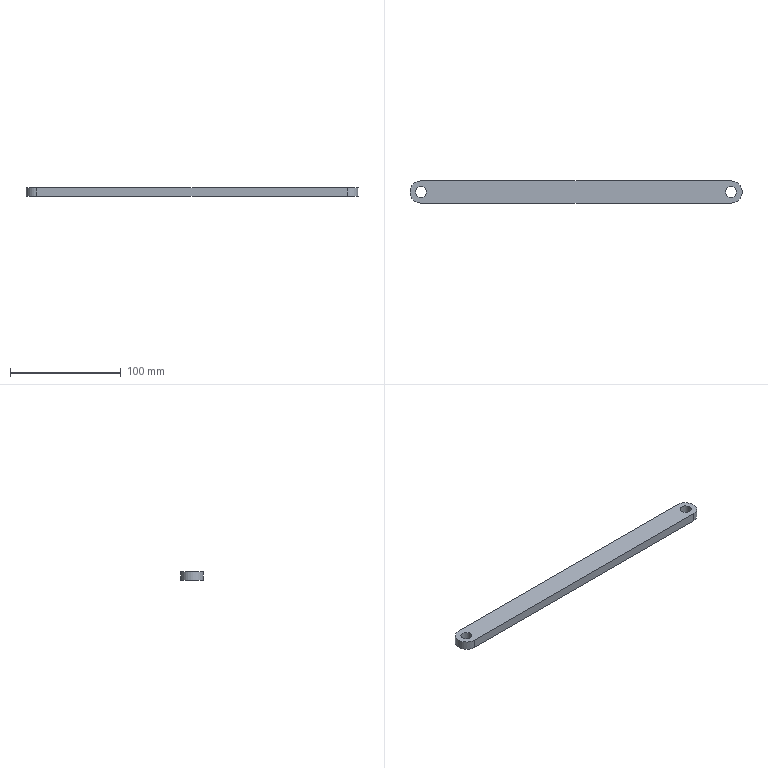Part | STEP file | tieqiangan | 1 solid | 8 faces | box 300 x 20 x 8 mm | volume 46057 mm3 | cylinder 4 | plane 4 | commonest cylinder face diameters 10 x2 20 x2
STEP:
#1=CARTESIAN_POINT('',(0.,0.,0.));
#2=DIRECTION('',(0.,0.,1.));
#3=DIRECTION('',(1.,0.,0.));
#4=AXIS2_PLACEMENT_3D('',#1,#2,#3);
#5=CARTESIAN_POINT('',(280.,10.,0.));
#6=VERTEX_POINT('',#5);
#7=CARTESIAN_POINT('',(280.,-10.,0.));
#8=VERTEX_POINT('',#7);
#9=CARTESIAN_POINT('',(280.,0.,0.));
#10=DIRECTION('',(0.,0.,-1.));
#11=DIRECTION('',(1.,0.,0.));
#12=AXIS2_PLACEMENT_3D('',#9,#10,#11);
#13=CIRCLE('',#12,10.);
#14=CARTESIAN_POINT('',(280.,0.,8.));
#15=DIRECTION('',(0.,0.,-1.));
#16=DIRECTION('',(-1.,0.,0.));
#17=AXIS2_PLACEMENT_3D('',#14,#15,#16);
#18=CYLINDRICAL_SURFACE('',#17,10.);
#19=CARTESIAN_POINT('',(-3.142,8.));
#20=DIRECTION('',(1.,0.));
#21=VECTOR('',#20,1.);
#22=LINE('',#19,#21);
#23=(GEOMETRIC_REPRESENTATION_CONTEXT(2)PARAMETRIC_REPRESENTATION_CONTEXT()REPRESENTATION_CONTEXT('',''));
#24=DEFINITIONAL_REPRESENTATION('',(#22),#23);
#25=PCURVE('',#18,#24);
#26=CARTESIAN_POINT('',(0.,0.,0.));
#27=DIRECTION('',(0.,0.,1.));
#28=DIRECTION('',(1.,0.,0.));
#29=AXIS2_PLACEMENT_3D('',#26,#27,#28);
#30=PLANE('',#29);
#31=CARTESIAN_POINT('',(290.,0.));
#32=CARTESIAN_POINT('',(290.,-17.321));
#33=CARTESIAN_POINT('',(275.,-8.66));
#34=CARTESIAN_POINT('',(260.,0.));
#35=CARTESIAN_POINT('',(275.,8.66));
#36=CARTESIAN_POINT('',(290.,17.321));
#37=CARTESIAN_POINT('',(290.,0.));
#38=(BOUNDED_CURVE()B_SPLINE_CURVE(2,(#31,#32,#33,#34,#35,#36,#37),.UNSPECIFIED.,.T.,.F.)B_SPLINE_CURVE_WITH_KNOTS((1,2,2,2,2,1),(-2.094,0.,2.094,4.189,6.283,8.378),.UNSPECIFIED.)CURVE()GEOMETRIC_REPRESENTATION_ITEM()RATIONAL_B_SPLINE_CURVE((1.,0.5,1.,0.5,1.,0.5,1.))REPRESENTATION_ITEM(''));
#39=(GEOMETRIC_REPRESENTATION_CONTEXT(2)PARAMETRIC_REPRESENTATION_CONTEXT()REPRESENTATION_CONTEXT('',''));
#40=DEFINITIONAL_REPRESENTATION('',(#38),#39);
#41=PCURVE('',#30,#40);
#42=SURFACE_CURVE('',#13,(#25,#41),.PCURVE_S1.);
#43=EDGE_CURVE('',#6,#8,#42,.T.);
#44=ORIENTED_EDGE('',*,*,#43,.F.);
#45=CARTESIAN_POINT('',(280.,10.,8.));
#46=VERTEX_POINT('',#45);
#47=CARTESIAN_POINT('',(280.,10.,8.));
#48=DIRECTION('',(0.,0.,-1.));
#49=VECTOR('',#48,1.);
#50=LINE('',#47,#49);
#51=CARTESIAN_POINT('',(1.571,0.));
#52=DIRECTION('',(0.,1.));
#53=VECTOR('',#52,1.);
#54=LINE('',#51,#53);
#55=(GEOMETRIC_REPRESENTATION_CONTEXT(2)PARAMETRIC_REPRESENTATION_CONTEXT()REPRESENTATION_CONTEXT('',''));
#56=DEFINITIONAL_REPRESENTATION('',(#54),#55);
#57=PCURVE('',#18,#56);
#58=CARTESIAN_POINT('',(0.,10.,8.));
#59=DIRECTION('',(0.,1.,0.));
#60=DIRECTION('',(-1.,0.,0.));
#61=AXIS2_PLACEMENT_3D('',#58,#59,#60);
#62=PLANE('',#61);
#63=CARTESIAN_POINT('',(-280.,0.));
#64=DIRECTION('',(0.,-1.));
#65=VECTOR('',#64,1.);
#66=LINE('',#63,#65);
#67=(GEOMETRIC_REPRESENTATION_CONTEXT(2)PARAMETRIC_REPRESENTATION_CONTEXT()REPRESENTATION_CONTEXT('',''));
#68=DEFINITIONAL_REPRESENTATION('',(#66),#67);
#69=PCURVE('',#62,#68);
#70=SURFACE_CURVE('',#50,(#57,#69),.PCURVE_S1.);
#71=EDGE_CURVE('',#46,#6,#70,.T.);
#72=ORIENTED_EDGE('',*,*,#71,.F.);
#73=CARTESIAN_POINT('',(280.,-10.,8.));
#74=VERTEX_POINT('',#73);
#75=CARTESIAN_POINT('',(280.,0.,8.));
#76=DIRECTION('',(0.,0.,-1.));
#77=DIRECTION('',(1.,0.,0.));
#78=AXIS2_PLACEMENT_3D('',#75,#76,#77);
#79=CIRCLE('',#78,10.);
#80=CARTESIAN_POINT('',(-3.142,0.));
#81=DIRECTION('',(1.,0.));
#82=VECTOR('',#81,1.);
#83=LINE('',#80,#82);
#84=(GEOMETRIC_REPRESENTATION_CONTEXT(2)PARAMETRIC_REPRESENTATION_CONTEXT()REPRESENTATION_CONTEXT('',''));
#85=DEFINITIONAL_REPRESENTATION('',(#83),#84);
#86=PCURVE('',#18,#85);
#87=CARTESIAN_POINT('',(0.,0.,8.));
#88=DIRECTION('',(0.,0.,1.));
#89=DIRECTION('',(1.,0.,0.));
#90=AXIS2_PLACEMENT_3D('',#87,#88,#89);
#91=PLANE('',#90);
#92=CARTESIAN_POINT('',(290.,0.));
#93=CARTESIAN_POINT('',(290.,-17.321));
#94=CARTESIAN_POINT('',(275.,-8.66));
#95=CARTESIAN_POINT('',(260.,0.));
#96=CARTESIAN_POINT('',(275.,8.66));
#97=CARTESIAN_POINT('',(290.,17.321));
#98=CARTESIAN_POINT('',(290.,0.));
#99=(BOUNDED_CURVE()B_SPLINE_CURVE(2,(#92,#93,#94,#95,#96,#97,#98),.UNSPECIFIED.,.T.,.F.)B_SPLINE_CURVE_WITH_KNOTS((1,2,2,2,2,1),(-2.094,0.,2.094,4.189,6.283,8.378),.UNSPECIFIED.)CURVE()GEOMETRIC_REPRESENTATION_ITEM()RATIONAL_B_SPLINE_CURVE((1.,0.5,1.,0.5,1.,0.5,1.))REPRESENTATION_ITEM(''));
#100=(GEOMETRIC_REPRESENTATION_CONTEXT(2)PARAMETRIC_REPRESENTATION_CONTEXT()REPRESENTATION_CONTEXT('',''));
#101=DEFINITIONAL_REPRESENTATION('',(#99),#100);
#102=PCURVE('',#91,#101);
#103=SURFACE_CURVE('',#79,(#86,#102),.PCURVE_S1.);
#104=EDGE_CURVE('',#46,#74,#103,.T.);
#105=ORIENTED_EDGE('',*,*,#104,.T.);
#106=CARTESIAN_POINT('',(280.,-10.,8.));
#107=DIRECTION('',(0.,0.,-1.));
#108=VECTOR('',#107,1.);
#109=LINE('',#106,#108);
#110=CARTESIAN_POINT('',(4.712,0.));
#111=DIRECTION('',(0.,1.));
#112=VECTOR('',#111,1.);
#113=LINE('',#110,#112);
#114=(GEOMETRIC_REPRESENTATION_CONTEXT(2)PARAMETRIC_REPRESENTATION_CONTEXT()REPRESENTATION_CONTEXT('',''));
#115=DEFINITIONAL_REPRESENTATION('',(#113),#114);
#116=PCURVE('',#18,#115);
#117=CARTESIAN_POINT('',(0.,-10.,8.));
#118=DIRECTION('',(0.,1.,0.));
#119=DIRECTION('',(-1.,0.,0.));
#120=AXIS2_PLACEMENT_3D('',#117,#118,#119);
#121=PLANE('',#120);
#122=CARTESIAN_POINT('',(-280.,0.));
#123=DIRECTION('',(0.,-1.));
#124=VECTOR('',#123,1.);
#125=LINE('',#122,#124);
#126=(GEOMETRIC_REPRESENTATION_CONTEXT(2)PARAMETRIC_REPRESENTATION_CONTEXT()REPRESENTATION_CONTEXT('',''));
#127=DEFINITIONAL_REPRESENTATION('',(#125),#126);
#128=PCURVE('',#121,#127);
#129=SURFACE_CURVE('',#109,(#116,#128),.PCURVE_S1.);
#130=EDGE_CURVE('',#74,#8,#129,.T.);
#131=ORIENTED_EDGE('',*,*,#130,.T.);
#132=EDGE_LOOP('',(#44,#72,#105,#131));
#133=FACE_BOUND('',#132,.T.);
#134=ADVANCED_FACE('',(#133),#18,.T.);
#135=CARTESIAN_POINT('',(0.,10.,0.));
#136=VERTEX_POINT('',#135);
#137=CARTESIAN_POINT('',(0.,10.,0.));
#138=DIRECTION('',(1.,0.,0.));
#139=VECTOR('',#138,1.);
#140=LINE('',#137,#139);
#141=CARTESIAN_POINT('',(0.,-8.));
#142=DIRECTION('',(-1.,0.));
#143=VECTOR('',#142,1.);
#144=LINE('',#141,#143);
#145=(GEOMETRIC_REPRESENTATION_CONTEXT(2)PARAMETRIC_REPRESENTATION_CONTEXT()REPRESENTATION_CONTEXT('',''));
#146=DEFINITIONAL_REPRESENTATION('',(#144),#145);
#147=PCURVE('',#62,#146);
#148=CARTESIAN_POINT('',(0.,10.));
#149=DIRECTION('',(1.,0.));
#150=VECTOR('',#149,1.);
#151=LINE('',#148,#150);
#152=(GEOMETRIC_REPRESENTATION_CONTEXT(2)PARAMETRIC_REPRESENTATION_CONTEXT()REPRESENTATION_CONTEXT('',''));
#153=DEFINITIONAL_REPRESENTATION('',(#151),#152);
#154=PCURVE('',#30,#153);
#155=SURFACE_CURVE('',#140,(#147,#154),.PCURVE_S1.);
#156=EDGE_CURVE('',#136,#6,#155,.T.);
#157=ORIENTED_EDGE('',*,*,#156,.F.);
#158=CARTESIAN_POINT('',(0.,10.,8.));
#159=VERTEX_POINT('',#158);
#160=CARTESIAN_POINT('',(0.,10.,8.));
#161=DIRECTION('',(0.,0.,-1.));
#162=VECTOR('',#161,1.);
#163=LINE('',#160,#162);
#164=CARTESIAN_POINT('',(0.,0.));
#165=DIRECTION('',(0.,-1.));
#166=VECTOR('',#165,1.);
#167=LINE('',#164,#166);
#168=(GEOMETRIC_REPRESENTATION_CONTEXT(2)PARAMETRIC_REPRESENTATION_CONTEXT()REPRESENTATION_CONTEXT('',''));
#169=DEFINITIONAL_REPRESENTATION('',(#167),#168);
#170=PCURVE('',#62,#169);
#171=CARTESIAN_POINT('',(0.,0.,8.));
#172=DIRECTION('',(0.,0.,-1.));
#173=DIRECTION('',(-1.,0.,0.));
#174=AXIS2_PLACEMENT_3D('',#171,#172,#173);
#175=CYLINDRICAL_SURFACE('',#174,10.);
#176=CARTESIAN_POINT('',(1.571,0.));
#177=DIRECTION('',(0.,1.));
#178=VECTOR('',#177,1.);
#179=LINE('',#176,#178);
#180=(GEOMETRIC_REPRESENTATION_CONTEXT(2)PARAMETRIC_REPRESENTATION_CONTEXT()REPRESENTATION_CONTEXT('',''));
#181=DEFINITIONAL_REPRESENTATION('',(#179),#180);
#182=PCURVE('',#175,#181);
#183=SURFACE_CURVE('',#163,(#170,#182),.PCURVE_S1.);
#184=EDGE_CURVE('',#159,#136,#183,.T.);
#185=ORIENTED_EDGE('',*,*,#184,.F.);
#186=CARTESIAN_POINT('',(0.,10.,8.));
#187=DIRECTION('',(1.,0.,0.));
#188=VECTOR('',#187,1.);
#189=LINE('',#186,#188);
#190=CARTESIAN_POINT('',(0.,0.));
#191=DIRECTION('',(-1.,0.));
#192=VECTOR('',#191,1.);
#193=LINE('',#190,#192);
#194=(GEOMETRIC_REPRESENTATION_CONTEXT(2)PARAMETRIC_REPRESENTATION_CONTEXT()REPRESENTATION_CONTEXT('',''));
#195=DEFINITIONAL_REPRESENTATION('',(#193),#194);
#196=PCURVE('',#62,#195);
#197=CARTESIAN_POINT('',(0.,10.));
#198=DIRECTION('',(1.,0.));
#199=VECTOR('',#198,1.);
#200=LINE('',#197,#199);
#201=(GEOMETRIC_REPRESENTATION_CONTEXT(2)PARAMETRIC_REPRESENTATION_CONTEXT()REPRESENTATION_CONTEXT('',''));
#202=DEFINITIONAL_REPRESENTATION('',(#200),#201);
#203=PCURVE('',#91,#202);
#204=SURFACE_CURVE('',#189,(#196,#203),.PCURVE_S1.);
#205=EDGE_CURVE('',#159,#46,#204,.T.);
#206=ORIENTED_EDGE('',*,*,#205,.T.);
#207=ORIENTED_EDGE('',*,*,#71,.T.);
#208=EDGE_LOOP('',(#157,#185,#206,#207));
#209=FACE_BOUND('',#208,.T.);
#210=ADVANCED_FACE('',(#209),#62,.T.);
#211=CARTESIAN_POINT('',(0.,-10.,0.));
#212=VERTEX_POINT('',#211);
#213=CARTESIAN_POINT('',(0.,0.,0.));
#214=DIRECTION('',(0.,0.,1.));
#215=DIRECTION('',(1.,0.,0.));
#216=AXIS2_PLACEMENT_3D('',#213,#214,#215);
#217=CIRCLE('',#216,10.);
#218=CARTESIAN_POINT('',(3.142,8.));
#219=DIRECTION('',(-1.,0.));
#220=VECTOR('',#219,1.);
#221=LINE('',#218,#220);
#222=(GEOMETRIC_REPRESENTATION_CONTEXT(2)PARAMETRIC_REPRESENTATION_CONTEXT()REPRESENTATION_CONTEXT('',''));
#223=DEFINITIONAL_REPRESENTATION('',(#221),#222);
#224=PCURVE('',#175,#223);
#225=CARTESIAN_POINT('',(0.,0.));
#226=DIRECTION('',(1.,0.));
#227=AXIS2_PLACEMENT_2D('',#225,#226);
#228=CIRCLE('',#227,10.);
#229=(GEOMETRIC_REPRESENTATION_CONTEXT(2)PARAMETRIC_REPRESENTATION_CONTEXT()REPRESENTATION_CONTEXT('',''));
#230=DEFINITIONAL_REPRESENTATION('',(#228),#229);
#231=PCURVE('',#30,#230);
#232=SURFACE_CURVE('',#217,(#224,#231),.PCURVE_S1.);
#233=EDGE_CURVE('',#136,#212,#232,.T.);
#234=ORIENTED_EDGE('',*,*,#233,.T.);
#235=CARTESIAN_POINT('',(0.,-10.,8.));
#236=VERTEX_POINT('',#235);
#237=CARTESIAN_POINT('',(0.,-10.,8.));
#238=DIRECTION('',(0.,0.,-1.));
#239=VECTOR('',#238,1.);
#240=LINE('',#237,#239);
#241=CARTESIAN_POINT('',(-1.571,0.));
#242=DIRECTION('',(0.,1.));
#243=VECTOR('',#242,1.);
#244=LINE('',#241,#243);
#245=(GEOMETRIC_REPRESENTATION_CONTEXT(2)PARAMETRIC_REPRESENTATION_CONTEXT()REPRESENTATION_CONTEXT('',''));
#246=DEFINITIONAL_REPRESENTATION('',(#244),#245);
#247=PCURVE('',#175,#246);
#248=CARTESIAN_POINT('',(0.,0.));
#249=DIRECTION('',(0.,-1.));
#250=VECTOR('',#249,1.);
#251=LINE('',#248,#250);
#252=(GEOMETRIC_REPRESENTATION_CONTEXT(2)PARAMETRIC_REPRESENTATION_CONTEXT()REPRESENTATION_CONTEXT('',''));
#253=DEFINITIONAL_REPRESENTATION('',(#251),#252);
#254=PCURVE('',#121,#253);
#255=SURFACE_CURVE('',#240,(#247,#254),.PCURVE_S1.);
#256=EDGE_CURVE('',#236,#212,#255,.T.);
#257=ORIENTED_EDGE('',*,*,#256,.F.);
#258=CARTESIAN_POINT('',(0.,0.,8.));
#259=DIRECTION('',(0.,0.,1.));
#260=DIRECTION('',(1.,0.,0.));
#261=AXIS2_PLACEMENT_3D('',#258,#259,#260);
#262=CIRCLE('',#261,10.);
#263=CARTESIAN_POINT('',(3.142,0.));
#264=DIRECTION('',(-1.,0.));
#265=VECTOR('',#264,1.);
#266=LINE('',#263,#265);
#267=(GEOMETRIC_REPRESENTATION_CONTEXT(2)PARAMETRIC_REPRESENTATION_CONTEXT()REPRESENTATION_CONTEXT('',''));
#268=DEFINITIONAL_REPRESENTATION('',(#266),#267);
#269=PCURVE('',#175,#268);
#270=CARTESIAN_POINT('',(0.,0.));
#271=DIRECTION('',(1.,0.));
#272=AXIS2_PLACEMENT_2D('',#270,#271);
#273=CIRCLE('',#272,10.);
#274=(GEOMETRIC_REPRESENTATION_CONTEXT(2)PARAMETRIC_REPRESENTATION_CONTEXT()REPRESENTATION_CONTEXT('',''));
#275=DEFINITIONAL_REPRESENTATION('',(#273),#274);
#276=PCURVE('',#91,#275);
#277=SURFACE_CURVE('',#262,(#269,#276),.PCURVE_S1.);
#278=EDGE_CURVE('',#159,#236,#277,.T.);
#279=ORIENTED_EDGE('',*,*,#278,.F.);
#280=ORIENTED_EDGE('',*,*,#184,.T.);
#281=EDGE_LOOP('',(#234,#257,#279,#280));
#282=FACE_BOUND('',#281,.T.);
#283=ADVANCED_FACE('',(#282),#175,.T.);
#284=CARTESIAN_POINT('',(0.,-10.,0.));
#285=DIRECTION('',(1.,0.,0.));
#286=VECTOR('',#285,1.);
#287=LINE('',#284,#286);
#288=CARTESIAN_POINT('',(0.,-8.));
#289=DIRECTION('',(-1.,0.));
#290=VECTOR('',#289,1.);
#291=LINE('',#288,#290);
#292=(GEOMETRIC_REPRESENTATION_CONTEXT(2)PARAMETRIC_REPRESENTATION_CONTEXT()REPRESENTATION_CONTEXT('',''));
#293=DEFINITIONAL_REPRESENTATION('',(#291),#292);
#294=PCURVE('',#121,#293);
#295=CARTESIAN_POINT('',(0.,-10.));
#296=DIRECTION('',(1.,0.));
#297=VECTOR('',#296,1.);
#298=LINE('',#295,#297);
#299=(GEOMETRIC_REPRESENTATION_CONTEXT(2)PARAMETRIC_REPRESENTATION_CONTEXT()REPRESENTATION_CONTEXT('',''));
#300=DEFINITIONAL_REPRESENTATION('',(#298),#299);
#301=PCURVE('',#30,#300);
#302=SURFACE_CURVE('',#287,(#294,#301),.PCURVE_S1.);
#303=EDGE_CURVE('',#212,#8,#302,.T.);
#304=ORIENTED_EDGE('',*,*,#303,.T.);
#305=ORIENTED_EDGE('',*,*,#130,.F.);
#306=CARTESIAN_POINT('',(0.,-10.,8.));
#307=DIRECTION('',(1.,0.,0.));
#308=VECTOR('',#307,1.);
#309=LINE('',#306,#308);
#310=CARTESIAN_POINT('',(0.,0.));
#311=DIRECTION('',(-1.,0.));
#312=VECTOR('',#311,1.);
#313=LINE('',#310,#312);
#314=(GEOMETRIC_REPRESENTATION_CONTEXT(2)PARAMETRIC_REPRESENTATION_CONTEXT()REPRESENTATION_CONTEXT('',''));
#315=DEFINITIONAL_REPRESENTATION('',(#313),#314);
#316=PCURVE('',#121,#315);
#317=CARTESIAN_POINT('',(0.,-10.));
#318=DIRECTION('',(1.,0.));
#319=VECTOR('',#318,1.);
#320=LINE('',#317,#319);
#321=(GEOMETRIC_REPRESENTATION_CONTEXT(2)PARAMETRIC_REPRESENTATION_CONTEXT()REPRESENTATION_CONTEXT('',''));
#322=DEFINITIONAL_REPRESENTATION('',(#320),#321);
#323=PCURVE('',#91,#322);
#324=SURFACE_CURVE('',#309,(#316,#323),.PCURVE_S1.);
#325=EDGE_CURVE('',#236,#74,#324,.T.);
#326=ORIENTED_EDGE('',*,*,#325,.F.);
#327=ORIENTED_EDGE('',*,*,#256,.T.);
#328=EDGE_LOOP('',(#304,#305,#326,#327));
#329=FACE_BOUND('',#328,.T.);
#330=ADVANCED_FACE('',(#329),#121,.F.);
#331=CARTESIAN_POINT('',(5.,0.,8.));
#332=VERTEX_POINT('',#331);
#333=CARTESIAN_POINT('',(0.,0.,8.));
#334=DIRECTION('',(0.,0.,1.));
#335=DIRECTION('',(1.,0.,0.));
#336=AXIS2_PLACEMENT_3D('',#333,#334,#335);
#337=CIRCLE('',#336,5.);
#338=CARTESIAN_POINT('',(0.,0.,8.));
#339=DIRECTION('',(0.,0.,-1.));
#340=DIRECTION('',(-1.,0.,0.));
#341=AXIS2_PLACEMENT_3D('',#338,#339,#340);
#342=CYLINDRICAL_SURFACE('',#341,5.);
#343=CARTESIAN_POINT('',(9.425,0.));
#344=DIRECTION('',(-1.,0.));
#345=VECTOR('',#344,1.);
#346=LINE('',#343,#345);
#347=(GEOMETRIC_REPRESENTATION_CONTEXT(2)PARAMETRIC_REPRESENTATION_CONTEXT()REPRESENTATION_CONTEXT('',''));
#348=DEFINITIONAL_REPRESENTATION('',(#346),#347);
#349=PCURVE('',#342,#348);
#350=CARTESIAN_POINT('',(0.,0.));
#351=DIRECTION('',(1.,0.));
#352=AXIS2_PLACEMENT_2D('',#350,#351);
#353=CIRCLE('',#352,5.);
#354=(GEOMETRIC_REPRESENTATION_CONTEXT(2)PARAMETRIC_REPRESENTATION_CONTEXT()REPRESENTATION_CONTEXT('',''));
#355=DEFINITIONAL_REPRESENTATION('',(#353),#354);
#356=PCURVE('',#91,#355);
#357=SURFACE_CURVE('',#337,(#349,#356),.PCURVE_S1.);
#358=EDGE_CURVE('',#332,#332,#357,.T.);
#359=ORIENTED_EDGE('',*,*,#358,.F.);
#360=CARTESIAN_POINT('',(5.,0.,0.));
#361=VERTEX_POINT('',#360);
#362=CARTESIAN_POINT('',(5.,0.,8.));
#363=CARTESIAN_POINT('',(5.,0.,0.));
#364=B_SPLINE_CURVE_WITH_KNOTS('',1,(#362,#363),.UNSPECIFIED.,.F.,.F.,(2,2),(0.,8.),.PIECEWISE_BEZIER_KNOTS.);
#365=CARTESIAN_POINT('',(9.425,0.));
#366=DIRECTION('',(0.,1.));
#367=VECTOR('',#366,1.);
#368=LINE('',#365,#367);
#369=(GEOMETRIC_REPRESENTATION_CONTEXT(2)PARAMETRIC_REPRESENTATION_CONTEXT()REPRESENTATION_CONTEXT('',''));
#370=DEFINITIONAL_REPRESENTATION('',(#368),#369);
#371=PCURVE('',#342,#370);
#372=CARTESIAN_POINT('',(3.142,0.));
#373=DIRECTION('',(0.,1.));
#374=VECTOR('',#373,1.);
#375=LINE('',#372,#374);
#376=(GEOMETRIC_REPRESENTATION_CONTEXT(2)PARAMETRIC_REPRESENTATION_CONTEXT()REPRESENTATION_CONTEXT('',''));
#377=DEFINITIONAL_REPRESENTATION('',(#375),#376);
#378=PCURVE('',#342,#377);
#379=SEAM_CURVE('',#364,(#371,#378),.PCURVE_S1.);
#380=EDGE_CURVE('',#332,#361,#379,.T.);
#381=ORIENTED_EDGE('',*,*,#380,.T.);
#382=CARTESIAN_POINT('',(0.,0.,0.));
#383=DIRECTION('',(0.,0.,1.));
#384=DIRECTION('',(1.,0.,0.));
#385=AXIS2_PLACEMENT_3D('',#382,#383,#384);
#386=CIRCLE('',#385,5.);
#387=CARTESIAN_POINT('',(9.425,8.));
#388=DIRECTION('',(-1.,0.));
#389=VECTOR('',#388,1.);
#390=LINE('',#387,#389);
#391=(GEOMETRIC_REPRESENTATION_CONTEXT(2)PARAMETRIC_REPRESENTATION_CONTEXT()REPRESENTATION_CONTEXT('',''));
#392=DEFINITIONAL_REPRESENTATION('',(#390),#391);
#393=PCURVE('',#342,#392);
#394=CARTESIAN_POINT('',(0.,0.));
#395=DIRECTION('',(1.,0.));
#396=AXIS2_PLACEMENT_2D('',#394,#395);
#397=CIRCLE('',#396,5.);
#398=(GEOMETRIC_REPRESENTATION_CONTEXT(2)PARAMETRIC_REPRESENTATION_CONTEXT()REPRESENTATION_CONTEXT('',''));
#399=DEFINITIONAL_REPRESENTATION('',(#397),#398);
#400=PCURVE('',#30,#399);
#401=SURFACE_CURVE('',#386,(#393,#400),.PCURVE_S1.);
#402=EDGE_CURVE('',#361,#361,#401,.T.);
#403=ORIENTED_EDGE('',*,*,#402,.T.);
#404=ORIENTED_EDGE('',*,*,#380,.F.);
#405=EDGE_LOOP('',(#359,#381,#403,#404));
#406=FACE_BOUND('',#405,.F.);
#407=ADVANCED_FACE('',(#406),#342,.F.);
#408=CARTESIAN_POINT('',(285.,0.,8.));
#409=VERTEX_POINT('',#408);
#410=CARTESIAN_POINT('',(280.,0.,8.));
#411=DIRECTION('',(0.,0.,-1.));
#412=DIRECTION('',(1.,0.,0.));
#413=AXIS2_PLACEMENT_3D('',#410,#411,#412);
#414=CIRCLE('',#413,5.);
#415=CARTESIAN_POINT('',(280.,0.,8.));
#416=DIRECTION('',(0.,0.,-1.));
#417=DIRECTION('',(-1.,0.,0.));
#418=AXIS2_PLACEMENT_3D('',#415,#416,#417);
#419=CYLINDRICAL_SURFACE('',#418,5.);
#420=CARTESIAN_POINT('',(3.142,0.));
#421=DIRECTION('',(1.,0.));
#422=VECTOR('',#421,1.);
#423=LINE('',#420,#422);
#424=(GEOMETRIC_REPRESENTATION_CONTEXT(2)PARAMETRIC_REPRESENTATION_CONTEXT()REPRESENTATION_CONTEXT('',''));
#425=DEFINITIONAL_REPRESENTATION('',(#423),#424);
#426=PCURVE('',#419,#425);
#427=CARTESIAN_POINT('',(285.,0.));
#428=CARTESIAN_POINT('',(285.,-8.66));
#429=CARTESIAN_POINT('',(277.5,-4.33));
#430=CARTESIAN_POINT('',(270.,0.));
#431=CARTESIAN_POINT('',(277.5,4.33));
#432=CARTESIAN_POINT('',(285.,8.66));
#433=CARTESIAN_POINT('',(285.,0.));
#434=(BOUNDED_CURVE()B_SPLINE_CURVE(2,(#427,#428,#429,#430,#431,#432,#433),.UNSPECIFIED.,.T.,.F.)B_SPLINE_CURVE_WITH_KNOTS((1,2,2,2,2,1),(-2.094,0.,2.094,4.189,6.283,8.378),.UNSPECIFIED.)CURVE()GEOMETRIC_REPRESENTATION_ITEM()RATIONAL_B_SPLINE_CURVE((1.,0.5,1.,0.5,1.,0.5,1.))REPRESENTATION_ITEM(''));
#435=(GEOMETRIC_REPRESENTATION_CONTEXT(2)PARAMETRIC_REPRESENTATION_CONTEXT()REPRESENTATION_CONTEXT('',''));
#436=DEFINITIONAL_REPRESENTATION('',(#434),#435);
#437=PCURVE('',#91,#436);
#438=SURFACE_CURVE('',#414,(#426,#437),.PCURVE_S1.);
#439=EDGE_CURVE('',#409,#409,#438,.T.);
#440=ORIENTED_EDGE('',*,*,#439,.T.);
#441=CARTESIAN_POINT('',(285.,0.,0.));
#442=VERTEX_POINT('',#441);
#443=CARTESIAN_POINT('',(285.,0.,8.));
#444=CARTESIAN_POINT('',(285.,0.,0.));
#445=B_SPLINE_CURVE_WITH_KNOTS('',1,(#443,#444),.UNSPECIFIED.,.F.,.F.,(2,2),(0.,8.),.PIECEWISE_BEZIER_KNOTS.);
#446=CARTESIAN_POINT('',(9.425,0.));
#447=DIRECTION('',(0.,1.));
#448=VECTOR('',#447,1.);
#449=LINE('',#446,#448);
#450=(GEOMETRIC_REPRESENTATION_CONTEXT(2)PARAMETRIC_REPRESENTATION_CONTEXT()REPRESENTATION_CONTEXT('',''));
#451=DEFINITIONAL_REPRESENTATION('',(#449),#450);
#452=PCURVE('',#419,#451);
#453=CARTESIAN_POINT('',(3.142,0.));
#454=DIRECTION('',(0.,1.));
#455=VECTOR('',#454,1.);
#456=LINE('',#453,#455);
#457=(GEOMETRIC_REPRESENTATION_CONTEXT(2)PARAMETRIC_REPRESENTATION_CONTEXT()REPRESENTATION_CONTEXT('',''));
#458=DEFINITIONAL_REPRESENTATION('',(#456),#457);
#459=PCURVE('',#419,#458);
#460=SEAM_CURVE('',#445,(#452,#459),.PCURVE_S1.);
#461=EDGE_CURVE('',#409,#442,#460,.T.);
#462=ORIENTED_EDGE('',*,*,#461,.T.);
#463=CARTESIAN_POINT('',(280.,0.,0.));
#464=DIRECTION('',(0.,0.,-1.));
#465=DIRECTION('',(1.,0.,0.));
#466=AXIS2_PLACEMENT_3D('',#463,#464,#465);
#467=CIRCLE('',#466,5.);
#468=CARTESIAN_POINT('',(3.142,8.));
#469=DIRECTION('',(1.,0.));
#470=VECTOR('',#469,1.);
#471=LINE('',#468,#470);
#472=(GEOMETRIC_REPRESENTATION_CONTEXT(2)PARAMETRIC_REPRESENTATION_CONTEXT()REPRESENTATION_CONTEXT('',''));
#473=DEFINITIONAL_REPRESENTATION('',(#471),#472);
#474=PCURVE('',#419,#473);
#475=CARTESIAN_POINT('',(285.,0.));
#476=CARTESIAN_POINT('',(285.,-8.66));
#477=CARTESIAN_POINT('',(277.5,-4.33));
#478=CARTESIAN_POINT('',(270.,0.));
#479=CARTESIAN_POINT('',(277.5,4.33));
#480=CARTESIAN_POINT('',(285.,8.66));
#481=CARTESIAN_POINT('',(285.,0.));
#482=(BOUNDED_CURVE()B_SPLINE_CURVE(2,(#475,#476,#477,#478,#479,#480,#481),.UNSPECIFIED.,.T.,.F.)B_SPLINE_CURVE_WITH_KNOTS((1,2,2,2,2,1),(-2.094,0.,2.094,4.189,6.283,8.378),.UNSPECIFIED.)CURVE()GEOMETRIC_REPRESENTATION_ITEM()RATIONAL_B_SPLINE_CURVE((1.,0.5,1.,0.5,1.,0.5,1.))REPRESENTATION_ITEM(''));
#483=(GEOMETRIC_REPRESENTATION_CONTEXT(2)PARAMETRIC_REPRESENTATION_CONTEXT()REPRESENTATION_CONTEXT('',''));
#484=DEFINITIONAL_REPRESENTATION('',(#482),#483);
#485=PCURVE('',#30,#484);
#486=SURFACE_CURVE('',#467,(#474,#485),.PCURVE_S1.);
#487=EDGE_CURVE('',#442,#442,#486,.T.);
#488=ORIENTED_EDGE('',*,*,#487,.F.);
#489=ORIENTED_EDGE('',*,*,#461,.F.);
#490=EDGE_LOOP('',(#440,#462,#488,#489));
#491=FACE_BOUND('',#490,.F.);
#492=ADVANCED_FACE('',(#491),#419,.F.);
#493=ORIENTED_EDGE('',*,*,#358,.F.);
#494=EDGE_LOOP('',(#493));
#495=FACE_BOUND('',#494,.T.);
#496=ORIENTED_EDGE('',*,*,#104,.F.);
#497=ORIENTED_EDGE('',*,*,#205,.F.);
#498=ORIENTED_EDGE('',*,*,#278,.T.);
#499=ORIENTED_EDGE('',*,*,#325,.T.);
#500=EDGE_LOOP('',(#496,#497,#498,#499));
#501=FACE_BOUND('',#500,.T.);
#502=ORIENTED_EDGE('',*,*,#439,.T.);
#503=EDGE_LOOP('',(#502));
#504=FACE_BOUND('',#503,.T.);
#505=ADVANCED_FACE('',(#495,#501,#504),#91,.T.);
#506=ORIENTED_EDGE('',*,*,#402,.T.);
#507=EDGE_LOOP('',(#506));
#508=FACE_BOUND('',#507,.T.);
#509=ORIENTED_EDGE('',*,*,#43,.T.);
#510=ORIENTED_EDGE('',*,*,#303,.F.);
#511=ORIENTED_EDGE('',*,*,#233,.F.);
#512=ORIENTED_EDGE('',*,*,#156,.T.);
#513=EDGE_LOOP('',(#509,#510,#511,#512));
#514=FACE_BOUND('',#513,.T.);
#515=ORIENTED_EDGE('',*,*,#487,.F.);
#516=EDGE_LOOP('',(#515));
#517=FACE_BOUND('',#516,.T.);
#518=ADVANCED_FACE('',(#508,#514,#517),#30,.F.);
#519=CLOSED_SHELL('',(#134,#210,#283,#330,#407,#492,#505,#518));
#520=MANIFOLD_SOLID_BREP('',#519);
#521=(LENGTH_UNIT()NAMED_UNIT(*)SI_UNIT(.MILLI.,.METRE.));
#522=UNCERTAINTY_MEASURE_WITH_UNIT(LENGTH_MEASURE(0.000002),#521,'','');
#523=(NAMED_UNIT(*)PLANE_ANGLE_UNIT()SI_UNIT($,.RADIAN.));
#524=(NAMED_UNIT(*)SI_UNIT($,.STERADIAN.)SOLID_ANGLE_UNIT());
#525=(GEOMETRIC_REPRESENTATION_CONTEXT(3)GLOBAL_UNCERTAINTY_ASSIGNED_CONTEXT((#522))GLOBAL_UNIT_ASSIGNED_CONTEXT((#521,#523,#524))REPRESENTATION_CONTEXT('',''));
#526=ADVANCED_BREP_SHAPE_REPRESENTATION('',(#4,#520),#525);